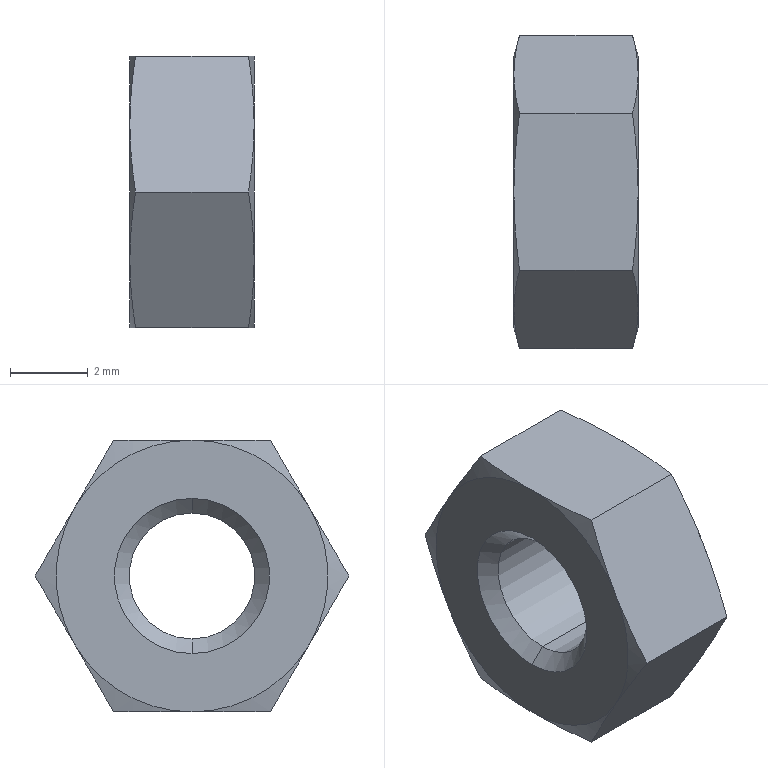Part | STEP file | 11-M4x0_7A11 | 1 solid | 26 faces | box 3.2 x 8.083 x 7 mm | volume 107.444 mm3 | cone 16 | plane 8 | cylinder 2 | commonest cylinder face diameters 3.242 x2
STEP:
#1=CARTESIAN_POINT('',(1.221,0.,-1.621));
#2=VERTEX_POINT('',#1);
#3=CARTESIAN_POINT('',(1.221,0.,1.621));
#4=VERTEX_POINT('',#3);
#5=CARTESIAN_POINT('',(1.221,0.,0.));
#6=DIRECTION('',(-1.,0.,0.));
#7=DIRECTION('',(0.,0.,1.));
#8=AXIS2_PLACEMENT_3D('',#5,#6,#7);
#9=CIRCLE('',#8,1.621);
#10=EDGE_CURVE('',#2,#4,#9,.T.);
#11=ORIENTED_EDGE('',*,*,#10,.T.);
#12=CARTESIAN_POINT('',(1.6,0.,2.));
#13=VERTEX_POINT('',#12);
#14=CARTESIAN_POINT('',(1.6,0.,2.));
#15=DIRECTION('',(0.7071,0.,0.7071));
#16=VECTOR('',#15,1000.);
#17=LINE('',#14,#16);
#18=EDGE_CURVE('',#4,#13,#17,.T.);
#19=ORIENTED_EDGE('',*,*,#18,.T.);
#20=CARTESIAN_POINT('',(1.6,0.,-2.));
#21=VERTEX_POINT('',#20);
#22=CARTESIAN_POINT('',(1.6,0.,0.));
#23=DIRECTION('',(-1.,0.,0.));
#24=DIRECTION('',(0.,0.,1.));
#25=AXIS2_PLACEMENT_3D('',#22,#23,#24);
#26=CIRCLE('',#25,2.);
#27=EDGE_CURVE('',#21,#13,#26,.T.);
#28=ORIENTED_EDGE('',*,*,#27,.F.);
#29=CARTESIAN_POINT('',(1.6,0.,-2.));
#30=DIRECTION('',(0.7071,0.,-0.7071));
#31=VECTOR('',#30,1000.);
#32=LINE('',#29,#31);
#33=EDGE_CURVE('',#2,#21,#32,.T.);
#34=ORIENTED_EDGE('',*,*,#33,.F.);
#35=EDGE_LOOP('',(#11,#19,#28,#34));
#36=FACE_OUTER_BOUND('',#35,.T.);
#37=CARTESIAN_POINT('',(1.6,0.,0.));
#38=DIRECTION('',(1.,0.,0.));
#39=DIRECTION('',(0.,0.,-1.));
#40=AXIS2_PLACEMENT_3D('',#37,#38,#39);
#41=CONICAL_SURFACE('',#40,2.,0.7854);
#42=ADVANCED_FACE('',(#36),#41,.F.);
#43=ORIENTED_EDGE('',*,*,#10,.F.);
#44=CARTESIAN_POINT('',(-1.221,0.,-1.621));
#45=VERTEX_POINT('',#44);
#46=CARTESIAN_POINT('',(1.6,0.,-1.621));
#47=DIRECTION('',(-1.,0.,0.));
#48=VECTOR('',#47,1000.);
#49=LINE('',#46,#48);
#50=EDGE_CURVE('',#2,#45,#49,.T.);
#51=ORIENTED_EDGE('',*,*,#50,.T.);
#52=CARTESIAN_POINT('',(-1.221,0.,1.621));
#53=VERTEX_POINT('',#52);
#54=CARTESIAN_POINT('',(-1.221,0.,0.));
#55=DIRECTION('',(-1.,0.,0.));
#56=DIRECTION('',(0.,0.,1.));
#57=AXIS2_PLACEMENT_3D('',#54,#55,#56);
#58=CIRCLE('',#57,1.621);
#59=EDGE_CURVE('',#45,#53,#58,.T.);
#60=ORIENTED_EDGE('',*,*,#59,.T.);
#61=CARTESIAN_POINT('',(1.6,0.,1.621));
#62=DIRECTION('',(-1.,0.,0.));
#63=VECTOR('',#62,1000.);
#64=LINE('',#61,#63);
#65=EDGE_CURVE('',#4,#53,#64,.T.);
#66=ORIENTED_EDGE('',*,*,#65,.F.);
#67=EDGE_LOOP('',(#43,#51,#60,#66));
#68=FACE_OUTER_BOUND('',#67,.T.);
#69=CARTESIAN_POINT('',(1.6,0.,0.));
#70=DIRECTION('',(-1.,0.,0.));
#71=DIRECTION('',(0.,0.,1.));
#72=AXIS2_PLACEMENT_3D('',#69,#70,#71);
#73=CYLINDRICAL_SURFACE('',#72,1.621);
#74=ADVANCED_FACE('',(#68),#73,.F.);
#75=ORIENTED_EDGE('',*,*,#59,.F.);
#76=CARTESIAN_POINT('',(-1.6,0.,-2.));
#77=VERTEX_POINT('',#76);
#78=CARTESIAN_POINT('',(-1.221,0.,-1.621));
#79=DIRECTION('',(-0.7071,0.,-0.7071));
#80=VECTOR('',#79,1000.);
#81=LINE('',#78,#80);
#82=EDGE_CURVE('',#45,#77,#81,.T.);
#83=ORIENTED_EDGE('',*,*,#82,.T.);
#84=CARTESIAN_POINT('',(-1.6,0.,2.));
#85=VERTEX_POINT('',#84);
#86=CARTESIAN_POINT('',(-1.6,0.,0.));
#87=DIRECTION('',(-1.,0.,0.));
#88=DIRECTION('',(0.,0.,1.));
#89=AXIS2_PLACEMENT_3D('',#86,#87,#88);
#90=CIRCLE('',#89,2.);
#91=EDGE_CURVE('',#77,#85,#90,.T.);
#92=ORIENTED_EDGE('',*,*,#91,.T.);
#93=CARTESIAN_POINT('',(-1.221,0.,1.621));
#94=DIRECTION('',(-0.7071,0.,0.7071));
#95=VECTOR('',#94,1000.);
#96=LINE('',#93,#95);
#97=EDGE_CURVE('',#53,#85,#96,.T.);
#98=ORIENTED_EDGE('',*,*,#97,.F.);
#99=EDGE_LOOP('',(#75,#83,#92,#98));
#100=FACE_OUTER_BOUND('',#99,.T.);
#101=CARTESIAN_POINT('',(-1.221,0.,0.));
#102=DIRECTION('',(-1.,0.,0.));
#103=DIRECTION('',(0.,0.,1.));
#104=AXIS2_PLACEMENT_3D('',#101,#102,#103);
#105=CONICAL_SURFACE('',#104,1.621,0.7854);
#106=ADVANCED_FACE('',(#100),#105,.F.);
#107=CARTESIAN_POINT('',(-1.6,-3.031,-1.75));
#108=VERTEX_POINT('',#107);
#109=CARTESIAN_POINT('',(-1.455,-4.041,0.));
#110=VERTEX_POINT('',#109);
#111=CARTESIAN_POINT('',(-1.6,-3.031,-1.75));
#112=CARTESIAN_POINT('',(-1.6,-3.368,-1.167));
#113=CARTESIAN_POINT('',(-1.545,-3.705,-0.5833));
#114=CARTESIAN_POINT('',(-1.455,-4.041,0.));
#115=B_SPLINE_CURVE_WITH_KNOTS('',3,(#111,#112,#113,#114),.UNSPECIFIED.,.F.,.F.,(4,4),(0.002021,0.004042),.UNSPECIFIED.);
#116=EDGE_CURVE('',#108,#110,#115,.T.);
#117=ORIENTED_EDGE('',*,*,#116,.T.);
#118=CARTESIAN_POINT('',(-1.6,-3.031,1.75));
#119=VERTEX_POINT('',#118);
#120=CARTESIAN_POINT('',(-1.455,-4.041,0.));
#121=CARTESIAN_POINT('',(-1.545,-3.705,0.5833));
#122=CARTESIAN_POINT('',(-1.6,-3.368,1.167));
#123=CARTESIAN_POINT('',(-1.6,-3.031,1.75));
#124=B_SPLINE_CURVE_WITH_KNOTS('',3,(#120,#121,#122,#123),.UNSPECIFIED.,.F.,.F.,(4,4),(0.000000231,0.002021),.UNSPECIFIED.);
#125=EDGE_CURVE('',#110,#119,#124,.T.);
#126=ORIENTED_EDGE('',*,*,#125,.T.);
#127=CARTESIAN_POINT('',(-1.6,0.,0.));
#128=DIRECTION('',(-1.,0.,0.));
#129=DIRECTION('',(0.,0.,1.));
#130=AXIS2_PLACEMENT_3D('',#127,#128,#129);
#131=CIRCLE('',#130,3.5);
#132=EDGE_CURVE('',#108,#119,#131,.T.);
#133=ORIENTED_EDGE('',*,*,#132,.F.);
#134=EDGE_LOOP('',(#117,#126,#133));
#135=FACE_OUTER_BOUND('',#134,.T.);
#136=CARTESIAN_POINT('',(-1.412,0.,0.));
#137=DIRECTION('',(1.,0.,0.));
#138=DIRECTION('',(0.,0.,-1.));
#139=AXIS2_PLACEMENT_3D('',#136,#137,#138);
#140=CONICAL_SURFACE('',#139,4.2,1.309);
#141=ADVANCED_FACE('',(#135),#140,.T.);
#142=CARTESIAN_POINT('',(-1.6,0.,3.5));
#143=VERTEX_POINT('',#142);
#144=CARTESIAN_POINT('',(-1.6,0.,0.));
#145=DIRECTION('',(-1.,0.,0.));
#146=DIRECTION('',(0.,0.,1.));
#147=AXIS2_PLACEMENT_3D('',#144,#145,#146);
#148=CIRCLE('',#147,3.5);
#149=EDGE_CURVE('',#119,#143,#148,.T.);
#150=ORIENTED_EDGE('',*,*,#149,.F.);
#151=CARTESIAN_POINT('',(-1.455,-2.021,3.5));
#152=VERTEX_POINT('',#151);
#153=CARTESIAN_POINT('',(-1.6,-3.031,1.75));
#154=CARTESIAN_POINT('',(-1.6,-2.694,2.333));
#155=CARTESIAN_POINT('',(-1.545,-2.358,2.917));
#156=CARTESIAN_POINT('',(-1.455,-2.021,3.5));
#157=B_SPLINE_CURVE_WITH_KNOTS('',3,(#153,#154,#155,#156),.UNSPECIFIED.,.F.,.F.,(4,4),(0.002021,0.004042),.UNSPECIFIED.);
#158=EDGE_CURVE('',#119,#152,#157,.T.);
#159=ORIENTED_EDGE('',*,*,#158,.T.);
#160=CARTESIAN_POINT('',(-1.455,-2.021,3.5));
#161=CARTESIAN_POINT('',(-1.545,-1.349,3.5));
#162=CARTESIAN_POINT('',(-1.6,-0.6726,3.5));
#163=CARTESIAN_POINT('',(-1.6,0.,3.5));
#164=B_SPLINE_CURVE_WITH_KNOTS('',3,(#160,#161,#162,#163),.UNSPECIFIED.,.F.,.F.,(4,4),(0.003384,0.005414),.UNSPECIFIED.);
#165=EDGE_CURVE('',#152,#143,#164,.T.);
#166=ORIENTED_EDGE('',*,*,#165,.T.);
#167=EDGE_LOOP('',(#150,#159,#166));
#168=FACE_OUTER_BOUND('',#167,.T.);
#169=CARTESIAN_POINT('',(-1.412,0.,0.));
#170=DIRECTION('',(1.,0.,0.));
#171=DIRECTION('',(0.,0.,-1.));
#172=AXIS2_PLACEMENT_3D('',#169,#170,#171);
#173=CONICAL_SURFACE('',#172,4.2,1.309);
#174=ADVANCED_FACE('',(#168),#173,.T.);
#175=CARTESIAN_POINT('',(-1.6,3.031,1.75));
#176=VERTEX_POINT('',#175);
#177=CARTESIAN_POINT('',(-1.6,0.,0.));
#178=DIRECTION('',(-1.,0.,0.));
#179=DIRECTION('',(0.,0.,1.));
#180=AXIS2_PLACEMENT_3D('',#177,#178,#179);
#181=CIRCLE('',#180,3.5);
#182=EDGE_CURVE('',#143,#176,#181,.T.);
#183=ORIENTED_EDGE('',*,*,#182,.F.);
#184=CARTESIAN_POINT('',(-1.455,2.021,3.5));
#185=VERTEX_POINT('',#184);
#186=CARTESIAN_POINT('',(-1.6,0.,3.5));
#187=CARTESIAN_POINT('',(-1.6,0.675,3.5));
#188=CARTESIAN_POINT('',(-1.545,1.348,3.5));
#189=CARTESIAN_POINT('',(-1.455,2.021,3.5));
#190=B_SPLINE_CURVE_WITH_KNOTS('',3,(#186,#187,#188,#189),.UNSPECIFIED.,.F.,.F.,(4,4),(0.005414,0.007452),.UNSPECIFIED.);
#191=EDGE_CURVE('',#143,#185,#190,.T.);
#192=ORIENTED_EDGE('',*,*,#191,.T.);
#193=CARTESIAN_POINT('',(-1.455,2.021,3.5));
#194=CARTESIAN_POINT('',(-1.545,2.358,2.917));
#195=CARTESIAN_POINT('',(-1.6,2.694,2.333));
#196=CARTESIAN_POINT('',(-1.6,3.031,1.75));
#197=B_SPLINE_CURVE_WITH_KNOTS('',3,(#193,#194,#195,#196),.UNSPECIFIED.,.F.,.F.,(4,4),(0.000000231,0.002021),.UNSPECIFIED.);
#198=EDGE_CURVE('',#185,#176,#197,.T.);
#199=ORIENTED_EDGE('',*,*,#198,.T.);
#200=EDGE_LOOP('',(#183,#192,#199));
#201=FACE_OUTER_BOUND('',#200,.T.);
#202=CARTESIAN_POINT('',(-1.412,0.,0.));
#203=DIRECTION('',(1.,0.,0.));
#204=DIRECTION('',(0.,0.,-1.));
#205=AXIS2_PLACEMENT_3D('',#202,#203,#204);
#206=CONICAL_SURFACE('',#205,4.2,1.309);
#207=ADVANCED_FACE('',(#201),#206,.T.);
#208=CARTESIAN_POINT('',(-1.6,0.,-3.5));
#209=VERTEX_POINT('',#208);
#210=CARTESIAN_POINT('',(-1.455,-2.021,-3.5));
#211=VERTEX_POINT('',#210);
#212=CARTESIAN_POINT('',(-1.6,0.,-3.5));
#213=CARTESIAN_POINT('',(-1.6,-0.6726,-3.5));
#214=CARTESIAN_POINT('',(-1.545,-1.349,-3.5));
#215=CARTESIAN_POINT('',(-1.455,-2.021,-3.5));
#216=B_SPLINE_CURVE_WITH_KNOTS('',3,(#212,#213,#214,#215),.UNSPECIFIED.,.F.,.F.,(4,4),(0.009728,0.01176),.UNSPECIFIED.);
#217=EDGE_CURVE('',#209,#211,#216,.T.);
#218=ORIENTED_EDGE('',*,*,#217,.T.);
#219=CARTESIAN_POINT('',(-1.455,-2.021,-3.5));
#220=CARTESIAN_POINT('',(-1.545,-2.358,-2.917));
#221=CARTESIAN_POINT('',(-1.6,-2.694,-2.333));
#222=CARTESIAN_POINT('',(-1.6,-3.031,-1.75));
#223=B_SPLINE_CURVE_WITH_KNOTS('',3,(#219,#220,#221,#222),.UNSPECIFIED.,.F.,.F.,(4,4),(0.000000231,0.002021),.UNSPECIFIED.);
#224=EDGE_CURVE('',#211,#108,#223,.T.);
#225=ORIENTED_EDGE('',*,*,#224,.T.);
#226=CARTESIAN_POINT('',(-1.6,0.,0.));
#227=DIRECTION('',(-1.,0.,0.));
#228=DIRECTION('',(0.,0.,1.));
#229=AXIS2_PLACEMENT_3D('',#226,#227,#228);
#230=CIRCLE('',#229,3.5);
#231=EDGE_CURVE('',#209,#108,#230,.T.);
#232=ORIENTED_EDGE('',*,*,#231,.F.);
#233=EDGE_LOOP('',(#218,#225,#232));
#234=FACE_OUTER_BOUND('',#233,.T.);
#235=CARTESIAN_POINT('',(-1.412,0.,0.));
#236=DIRECTION('',(1.,0.,0.));
#237=DIRECTION('',(0.,0.,-1.));
#238=AXIS2_PLACEMENT_3D('',#235,#236,#237);
#239=CONICAL_SURFACE('',#238,4.2,1.309);
#240=ADVANCED_FACE('',(#234),#239,.T.);
#241=CARTESIAN_POINT('',(-1.6,3.031,-1.75));
#242=VERTEX_POINT('',#241);
#243=CARTESIAN_POINT('',(-1.6,0.,0.));
#244=DIRECTION('',(-1.,0.,0.));
#245=DIRECTION('',(0.,0.,1.));
#246=AXIS2_PLACEMENT_3D('',#243,#244,#245);
#247=CIRCLE('',#246,3.5);
#248=EDGE_CURVE('',#176,#242,#247,.T.);
#249=ORIENTED_EDGE('',*,*,#248,.F.);
#250=CARTESIAN_POINT('',(-1.455,4.041,0.));
#251=VERTEX_POINT('',#250);
#252=CARTESIAN_POINT('',(-1.6,3.031,1.75));
#253=CARTESIAN_POINT('',(-1.6,3.368,1.167));
#254=CARTESIAN_POINT('',(-1.545,3.705,0.5833));
#255=CARTESIAN_POINT('',(-1.455,4.041,0.));
#256=B_SPLINE_CURVE_WITH_KNOTS('',3,(#252,#253,#254,#255),.UNSPECIFIED.,.F.,.F.,(4,4),(0.002021,0.004042),.UNSPECIFIED.);
#257=EDGE_CURVE('',#176,#251,#256,.T.);
#258=ORIENTED_EDGE('',*,*,#257,.T.);
#259=CARTESIAN_POINT('',(-1.455,4.041,0.));
#260=CARTESIAN_POINT('',(-1.545,3.705,-0.5833));
#261=CARTESIAN_POINT('',(-1.6,3.368,-1.167));
#262=CARTESIAN_POINT('',(-1.6,3.031,-1.75));
#263=B_SPLINE_CURVE_WITH_KNOTS('',3,(#259,#260,#261,#262),.UNSPECIFIED.,.F.,.F.,(4,4),(0.000000231,0.002021),.UNSPECIFIED.);
#264=EDGE_CURVE('',#251,#242,#263,.T.);
#265=ORIENTED_EDGE('',*,*,#264,.T.);
#266=EDGE_LOOP('',(#249,#258,#265));
#267=FACE_OUTER_BOUND('',#266,.T.);
#268=CARTESIAN_POINT('',(-1.412,0.,0.));
#269=DIRECTION('',(1.,0.,0.));
#270=DIRECTION('',(0.,0.,-1.));
#271=AXIS2_PLACEMENT_3D('',#268,#269,#270);
#272=CONICAL_SURFACE('',#271,4.2,1.309);
#273=ADVANCED_FACE('',(#267),#272,.T.);
#274=CARTESIAN_POINT('',(1.6,3.031,-1.75));
#275=VERTEX_POINT('',#274);
#276=CARTESIAN_POINT('',(1.455,4.041,0.));
#277=VERTEX_POINT('',#276);
#278=CARTESIAN_POINT('',(1.6,3.031,-1.75));
#279=CARTESIAN_POINT('',(1.6,3.368,-1.167));
#280=CARTESIAN_POINT('',(1.545,3.705,-0.5833));
#281=CARTESIAN_POINT('',(1.455,4.041,0.));
#282=B_SPLINE_CURVE_WITH_KNOTS('',3,(#278,#279,#280,#281),.UNSPECIFIED.,.F.,.F.,(4,4),(0.002021,0.004042),.UNSPECIFIED.);
#283=EDGE_CURVE('',#275,#277,#282,.T.);
#284=ORIENTED_EDGE('',*,*,#283,.T.);
#285=CARTESIAN_POINT('',(1.6,3.031,1.75));
#286=VERTEX_POINT('',#285);
#287=CARTESIAN_POINT('',(1.455,4.041,0.));
#288=CARTESIAN_POINT('',(1.545,3.705,0.5833));
#289=CARTESIAN_POINT('',(1.6,3.368,1.167));
#290=CARTESIAN_POINT('',(1.6,3.031,1.75));
#291=B_SPLINE_CURVE_WITH_KNOTS('',3,(#287,#288,#289,#290),.UNSPECIFIED.,.F.,.F.,(4,4),(0.000000231,0.002021),.UNSPECIFIED.);
#292=EDGE_CURVE('',#277,#286,#291,.T.);
#293=ORIENTED_EDGE('',*,*,#292,.T.);
#294=CARTESIAN_POINT('',(1.6,0.,0.));
#295=DIRECTION('',(-1.,0.,0.));
#296=DIRECTION('',(0.,0.,1.));
#297=AXIS2_PLACEMENT_3D('',#294,#295,#296);
#298=CIRCLE('',#297,3.5);
#299=EDGE_CURVE('',#286,#275,#298,.T.);
#300=ORIENTED_EDGE('',*,*,#299,.T.);
#301=EDGE_LOOP('',(#284,#293,#300));
#302=FACE_OUTER_BOUND('',#301,.T.);
#303=CARTESIAN_POINT('',(1.6,0.,0.));
#304=DIRECTION('',(-1.,0.,0.));
#305=DIRECTION('',(0.,0.,1.));
#306=AXIS2_PLACEMENT_3D('',#303,#304,#305);
#307=CONICAL_SURFACE('',#306,3.5,1.309);
#308=ADVANCED_FACE('',(#302),#307,.T.);
#309=CARTESIAN_POINT('',(1.6,0.,3.5));
#310=VERTEX_POINT('',#309);
#311=CARTESIAN_POINT('',(1.6,0.,0.));
#312=DIRECTION('',(-1.,0.,0.));
#313=DIRECTION('',(0.,0.,1.));
#314=AXIS2_PLACEMENT_3D('',#311,#312,#313);
#315=CIRCLE('',#314,3.5);
#316=EDGE_CURVE('',#310,#286,#315,.T.);
#317=ORIENTED_EDGE('',*,*,#316,.T.);
#318=CARTESIAN_POINT('',(1.455,2.021,3.5));
#319=VERTEX_POINT('',#318);
#320=CARTESIAN_POINT('',(1.6,3.031,1.75));
#321=CARTESIAN_POINT('',(1.6,2.694,2.333));
#322=CARTESIAN_POINT('',(1.545,2.358,2.917));
#323=CARTESIAN_POINT('',(1.455,2.021,3.5));
#324=B_SPLINE_CURVE_WITH_KNOTS('',3,(#320,#321,#322,#323),.UNSPECIFIED.,.F.,.F.,(4,4),(0.002021,0.004042),.UNSPECIFIED.);
#325=EDGE_CURVE('',#286,#319,#324,.T.);
#326=ORIENTED_EDGE('',*,*,#325,.T.);
#327=CARTESIAN_POINT('',(1.455,2.021,3.5));
#328=CARTESIAN_POINT('',(1.545,1.348,3.5));
#329=CARTESIAN_POINT('',(1.6,0.675,3.5));
#330=CARTESIAN_POINT('',(1.6,0.,3.5));
#331=B_SPLINE_CURVE_WITH_KNOTS('',3,(#327,#328,#329,#330),.UNSPECIFIED.,.F.,.F.,(4,4),(0.007694,0.009728),.UNSPECIFIED.);
#332=EDGE_CURVE('',#319,#310,#331,.T.);
#333=ORIENTED_EDGE('',*,*,#332,.T.);
#334=EDGE_LOOP('',(#317,#326,#333));
#335=FACE_OUTER_BOUND('',#334,.T.);
#336=CARTESIAN_POINT('',(1.6,0.,0.));
#337=DIRECTION('',(-1.,0.,0.));
#338=DIRECTION('',(0.,0.,1.));
#339=AXIS2_PLACEMENT_3D('',#336,#337,#338);
#340=CONICAL_SURFACE('',#339,3.5,1.309);
#341=ADVANCED_FACE('',(#335),#340,.T.);
#342=CARTESIAN_POINT('',(1.6,-3.031,1.75));
#343=VERTEX_POINT('',#342);
#344=CARTESIAN_POINT('',(1.6,0.,0.));
#345=DIRECTION('',(-1.,0.,0.));
#346=DIRECTION('',(0.,0.,1.));
#347=AXIS2_PLACEMENT_3D('',#344,#345,#346);
#348=CIRCLE('',#347,3.5);
#349=EDGE_CURVE('',#343,#310,#348,.T.);
#350=ORIENTED_EDGE('',*,*,#349,.T.);
#351=CARTESIAN_POINT('',(1.455,-2.021,3.5));
#352=VERTEX_POINT('',#351);
#353=CARTESIAN_POINT('',(1.6,0.,3.5));
#354=CARTESIAN_POINT('',(1.6,-0.6726,3.5));
#355=CARTESIAN_POINT('',(1.545,-1.349,3.5));
#356=CARTESIAN_POINT('',(1.455,-2.021,3.5));
#357=B_SPLINE_CURVE_WITH_KNOTS('',3,(#353,#354,#355,#356),.UNSPECIFIED.,.F.,.F.,(4,4),(0.009728,0.01176),.UNSPECIFIED.);
#358=EDGE_CURVE('',#310,#352,#357,.T.);
#359=ORIENTED_EDGE('',*,*,#358,.T.);
#360=CARTESIAN_POINT('',(1.455,-2.021,3.5));
#361=CARTESIAN_POINT('',(1.545,-2.358,2.917));
#362=CARTESIAN_POINT('',(1.6,-2.694,2.333));
#363=CARTESIAN_POINT('',(1.6,-3.031,1.75));
#364=B_SPLINE_CURVE_WITH_KNOTS('',3,(#360,#361,#362,#363),.UNSPECIFIED.,.F.,.F.,(4,4),(0.000000231,0.002021),.UNSPECIFIED.);
#365=EDGE_CURVE('',#352,#343,#364,.T.);
#366=ORIENTED_EDGE('',*,*,#365,.T.);
#367=EDGE_LOOP('',(#350,#359,#366));
#368=FACE_OUTER_BOUND('',#367,.T.);
#369=CARTESIAN_POINT('',(1.6,0.,0.));
#370=DIRECTION('',(-1.,0.,0.));
#371=DIRECTION('',(0.,0.,1.));
#372=AXIS2_PLACEMENT_3D('',#369,#370,#371);
#373=CONICAL_SURFACE('',#372,3.5,1.309);
#374=ADVANCED_FACE('',(#368),#373,.T.);
#375=CARTESIAN_POINT('',(1.6,-3.031,-1.75));
#376=VERTEX_POINT('',#375);
#377=CARTESIAN_POINT('',(1.6,0.,0.));
#378=DIRECTION('',(-1.,0.,0.));
#379=DIRECTION('',(0.,0.,1.));
#380=AXIS2_PLACEMENT_3D('',#377,#378,#379);
#381=CIRCLE('',#380,3.5);
#382=EDGE_CURVE('',#376,#343,#381,.T.);
#383=ORIENTED_EDGE('',*,*,#382,.T.);
#384=CARTESIAN_POINT('',(1.455,-4.041,0.));
#385=VERTEX_POINT('',#384);
#386=CARTESIAN_POINT('',(1.6,-3.031,1.75));
#387=CARTESIAN_POINT('',(1.6,-3.368,1.167));
#388=CARTESIAN_POINT('',(1.545,-3.705,0.5833));
#389=CARTESIAN_POINT('',(1.455,-4.041,0.));
#390=B_SPLINE_CURVE_WITH_KNOTS('',3,(#386,#387,#388,#389),.UNSPECIFIED.,.F.,.F.,(4,4),(0.002021,0.004042),.UNSPECIFIED.);
#391=EDGE_CURVE('',#343,#385,#390,.T.);
#392=ORIENTED_EDGE('',*,*,#391,.T.);
#393=CARTESIAN_POINT('',(1.455,-4.041,0.));
#394=CARTESIAN_POINT('',(1.545,-3.705,-0.5833));
#395=CARTESIAN_POINT('',(1.6,-3.368,-1.167));
#396=CARTESIAN_POINT('',(1.6,-3.031,-1.75));
#397=B_SPLINE_CURVE_WITH_KNOTS('',3,(#393,#394,#395,#396),.UNSPECIFIED.,.F.,.F.,(4,4),(0.000000231,0.002021),.UNSPECIFIED.);
#398=EDGE_CURVE('',#385,#376,#397,.T.);
#399=ORIENTED_EDGE('',*,*,#398,.T.);
#400=EDGE_LOOP('',(#383,#392,#399));
#401=FACE_OUTER_BOUND('',#400,.T.);
#402=CARTESIAN_POINT('',(1.6,0.,0.));
#403=DIRECTION('',(-1.,0.,0.));
#404=DIRECTION('',(0.,0.,1.));
#405=AXIS2_PLACEMENT_3D('',#402,#403,#404);
#406=CONICAL_SURFACE('',#405,3.5,1.309);
#407=ADVANCED_FACE('',(#401),#406,.T.);
#408=CARTESIAN_POINT('',(1.6,0.,-3.5));
#409=VERTEX_POINT('',#408);
#410=CARTESIAN_POINT('',(1.6,0.,0.));
#411=DIRECTION('',(-1.,0.,0.));
#412=DIRECTION('',(0.,0.,1.));
#413=AXIS2_PLACEMENT_3D('',#410,#411,#412);
#414=CIRCLE('',#413,3.5);
#415=EDGE_CURVE('',#409,#376,#414,.T.);
#416=ORIENTED_EDGE('',*,*,#415,.T.);
#417=CARTESIAN_POINT('',(1.455,-2.021,-3.5));
#418=VERTEX_POINT('',#417);
#419=CARTESIAN_POINT('',(1.6,-3.031,-1.75));
#420=CARTESIAN_POINT('',(1.6,-2.694,-2.333));
#421=CARTESIAN_POINT('',(1.545,-2.358,-2.917));
#422=CARTESIAN_POINT('',(1.455,-2.021,-3.5));
#423=B_SPLINE_CURVE_WITH_KNOTS('',3,(#419,#420,#421,#422),.UNSPECIFIED.,.F.,.F.,(4,4),(0.002021,0.004042),.UNSPECIFIED.);
#424=EDGE_CURVE('',#376,#418,#423,.T.);
#425=ORIENTED_EDGE('',*,*,#424,.T.);
#426=CARTESIAN_POINT('',(1.455,-2.021,-3.5));
#427=CARTESIAN_POINT('',(1.545,-1.349,-3.5));
#428=CARTESIAN_POINT('',(1.6,-0.6726,-3.5));
#429=CARTESIAN_POINT('',(1.6,0.,-3.5));
#430=B_SPLINE_CURVE_WITH_KNOTS('',3,(#426,#427,#428,#429),.UNSPECIFIED.,.F.,.F.,(4,4),(0.003384,0.005414),.UNSPECIFIED.);
#431=EDGE_CURVE('',#418,#409,#430,.T.);
#432=ORIENTED_EDGE('',*,*,#431,.T.);
#433=EDGE_LOOP('',(#416,#425,#432));
#434=FACE_OUTER_BOUND('',#433,.T.);
#435=CARTESIAN_POINT('',(1.6,0.,0.));
#436=DIRECTION('',(-1.,0.,0.));
#437=DIRECTION('',(0.,0.,1.));
#438=AXIS2_PLACEMENT_3D('',#435,#436,#437);
#439=CONICAL_SURFACE('',#438,3.5,1.309);
#440=ADVANCED_FACE('',(#434),#439,.T.);
#441=ORIENTED_EDGE('',*,*,#182,.T.);
#442=ORIENTED_EDGE('',*,*,#248,.T.);
#443=CARTESIAN_POINT('',(-1.6,0.,0.));
#444=DIRECTION('',(-1.,0.,0.));
#445=DIRECTION('',(0.,0.,1.));
#446=AXIS2_PLACEMENT_3D('',#443,#444,#445);
#447=CIRCLE('',#446,3.5);
#448=EDGE_CURVE('',#242,#209,#447,.T.);
#449=ORIENTED_EDGE('',*,*,#448,.T.);
#450=ORIENTED_EDGE('',*,*,#231,.T.);
#451=ORIENTED_EDGE('',*,*,#132,.T.);
#452=ORIENTED_EDGE('',*,*,#149,.T.);
#453=EDGE_LOOP('',(#441,#442,#449,#450,#451,#452));
#454=FACE_OUTER_BOUND('',#453,.T.);
#455=CARTESIAN_POINT('',(-1.6,0.,0.));
#456=DIRECTION('',(-1.,0.,0.));
#457=DIRECTION('',(0.,0.,1.));
#458=AXIS2_PLACEMENT_3D('',#455,#456,#457);
#459=CIRCLE('',#458,2.);
#460=EDGE_CURVE('',#85,#77,#459,.T.);
#461=ORIENTED_EDGE('',*,*,#460,.F.);
#462=ORIENTED_EDGE('',*,*,#91,.F.);
#463=EDGE_LOOP('',(#461,#462));
#464=FACE_BOUND('',#463,.T.);
#465=CARTESIAN_POINT('',(-1.6,0.,0.));
#466=DIRECTION('',(1.,0.,0.));
#467=DIRECTION('',(0.,0.,-1.));
#468=AXIS2_PLACEMENT_3D('',#465,#466,#467);
#469=PLANE('',#468);
#470=ADVANCED_FACE('',(#454,#464),#469,.F.);
#471=ORIENTED_EDGE('',*,*,#316,.F.);
#472=ORIENTED_EDGE('',*,*,#349,.F.);
#473=ORIENTED_EDGE('',*,*,#382,.F.);
#474=ORIENTED_EDGE('',*,*,#415,.F.);
#475=CARTESIAN_POINT('',(1.6,0.,0.));
#476=DIRECTION('',(-1.,0.,0.));
#477=DIRECTION('',(0.,0.,1.));
#478=AXIS2_PLACEMENT_3D('',#475,#476,#477);
#479=CIRCLE('',#478,3.5);
#480=EDGE_CURVE('',#275,#409,#479,.T.);
#481=ORIENTED_EDGE('',*,*,#480,.F.);
#482=ORIENTED_EDGE('',*,*,#299,.F.);
#483=EDGE_LOOP('',(#471,#472,#473,#474,#481,#482));
#484=FACE_OUTER_BOUND('',#483,.T.);
#485=ORIENTED_EDGE('',*,*,#27,.T.);
#486=CARTESIAN_POINT('',(1.6,0.,0.));
#487=DIRECTION('',(-1.,0.,0.));
#488=DIRECTION('',(0.,0.,1.));
#489=AXIS2_PLACEMENT_3D('',#486,#487,#488);
#490=CIRCLE('',#489,2.);
#491=EDGE_CURVE('',#13,#21,#490,.T.);
#492=ORIENTED_EDGE('',*,*,#491,.T.);
#493=EDGE_LOOP('',(#485,#492));
#494=FACE_BOUND('',#493,.T.);
#495=CARTESIAN_POINT('',(1.6,3.5,0.));
#496=DIRECTION('',(-1.,0.,0.));
#497=DIRECTION('',(0.,0.,1.));
#498=AXIS2_PLACEMENT_3D('',#495,#496,#497);
#499=PLANE('',#498);
#500=ADVANCED_FACE('',(#484,#494),#499,.F.);
#501=CARTESIAN_POINT('',(-1.455,2.021,-3.5));
#502=VERTEX_POINT('',#501);
#503=CARTESIAN_POINT('',(-1.6,3.031,-1.75));
#504=CARTESIAN_POINT('',(-1.6,2.694,-2.333));
#505=CARTESIAN_POINT('',(-1.545,2.358,-2.917));
#506=CARTESIAN_POINT('',(-1.455,2.021,-3.5));
#507=B_SPLINE_CURVE_WITH_KNOTS('',3,(#503,#504,#505,#506),.UNSPECIFIED.,.F.,.F.,(4,4),(0.002021,0.004042),.UNSPECIFIED.);
#508=EDGE_CURVE('',#242,#502,#507,.T.);
#509=ORIENTED_EDGE('',*,*,#508,.T.);
#510=CARTESIAN_POINT('',(-1.455,2.021,-3.5));
#511=CARTESIAN_POINT('',(-1.545,1.348,-3.5));
#512=CARTESIAN_POINT('',(-1.6,0.675,-3.5));
#513=CARTESIAN_POINT('',(-1.6,0.,-3.5));
#514=B_SPLINE_CURVE_WITH_KNOTS('',3,(#510,#511,#512,#513),.UNSPECIFIED.,.F.,.F.,(4,4),(0.007694,0.009728),.UNSPECIFIED.);
#515=EDGE_CURVE('',#502,#209,#514,.T.);
#516=ORIENTED_EDGE('',*,*,#515,.T.);
#517=ORIENTED_EDGE('',*,*,#448,.F.);
#518=EDGE_LOOP('',(#509,#516,#517));
#519=FACE_OUTER_BOUND('',#518,.T.);
#520=CARTESIAN_POINT('',(-1.412,0.,0.));
#521=DIRECTION('',(1.,0.,0.));
#522=DIRECTION('',(0.,0.,-1.));
#523=AXIS2_PLACEMENT_3D('',#520,#521,#522);
#524=CONICAL_SURFACE('',#523,4.2,1.309);
#525=ADVANCED_FACE('',(#519),#524,.T.);
#526=ORIENTED_EDGE('',*,*,#480,.T.);
#527=CARTESIAN_POINT('',(1.455,2.021,-3.5));
#528=VERTEX_POINT('',#527);
#529=CARTESIAN_POINT('',(1.6,0.,-3.5));
#530=CARTESIAN_POINT('',(1.6,0.675,-3.5));
#531=CARTESIAN_POINT('',(1.545,1.348,-3.5));
#532=CARTESIAN_POINT('',(1.455,2.021,-3.5));
#533=B_SPLINE_CURVE_WITH_KNOTS('',3,(#529,#530,#531,#532),.UNSPECIFIED.,.F.,.F.,(4,4),(0.005414,0.007452),.UNSPECIFIED.);
#534=EDGE_CURVE('',#409,#528,#533,.T.);
#535=ORIENTED_EDGE('',*,*,#534,.T.);
#536=CARTESIAN_POINT('',(1.455,2.021,-3.5));
#537=CARTESIAN_POINT('',(1.545,2.358,-2.917));
#538=CARTESIAN_POINT('',(1.6,2.694,-2.333));
#539=CARTESIAN_POINT('',(1.6,3.031,-1.75));
#540=B_SPLINE_CURVE_WITH_KNOTS('',3,(#536,#537,#538,#539),.UNSPECIFIED.,.F.,.F.,(4,4),(0.000000231,0.002021),.UNSPECIFIED.);
#541=EDGE_CURVE('',#528,#275,#540,.T.);
#542=ORIENTED_EDGE('',*,*,#541,.T.);
#543=EDGE_LOOP('',(#526,#535,#542));
#544=FACE_OUTER_BOUND('',#543,.T.);
#545=CARTESIAN_POINT('',(1.6,0.,0.));
#546=DIRECTION('',(-1.,0.,0.));
#547=DIRECTION('',(0.,0.,1.));
#548=AXIS2_PLACEMENT_3D('',#545,#546,#547);
#549=CONICAL_SURFACE('',#548,3.5,1.309);
#550=ADVANCED_FACE('',(#544),#549,.T.);
#551=ORIENTED_EDGE('',*,*,#82,.F.);
#552=CARTESIAN_POINT('',(-1.221,0.,0.));
#553=DIRECTION('',(-1.,0.,0.));
#554=DIRECTION('',(0.,0.,1.));
#555=AXIS2_PLACEMENT_3D('',#552,#553,#554);
#556=CIRCLE('',#555,1.621);
#557=EDGE_CURVE('',#53,#45,#556,.T.);
#558=ORIENTED_EDGE('',*,*,#557,.F.);
#559=ORIENTED_EDGE('',*,*,#97,.T.);
#560=ORIENTED_EDGE('',*,*,#460,.T.);
#561=EDGE_LOOP('',(#551,#558,#559,#560));
#562=FACE_OUTER_BOUND('',#561,.T.);
#563=CARTESIAN_POINT('',(-1.221,0.,0.));
#564=DIRECTION('',(-1.,0.,0.));
#565=DIRECTION('',(0.,0.,1.));
#566=AXIS2_PLACEMENT_3D('',#563,#564,#565);
#567=CONICAL_SURFACE('',#566,1.621,0.7854);
#568=ADVANCED_FACE('',(#562),#567,.F.);
#569=ORIENTED_EDGE('',*,*,#50,.F.);
#570=CARTESIAN_POINT('',(1.221,0.,0.));
#571=DIRECTION('',(-1.,0.,0.));
#572=DIRECTION('',(0.,0.,1.));
#573=AXIS2_PLACEMENT_3D('',#570,#571,#572);
#574=CIRCLE('',#573,1.621);
#575=EDGE_CURVE('',#4,#2,#574,.T.);
#576=ORIENTED_EDGE('',*,*,#575,.F.);
#577=ORIENTED_EDGE('',*,*,#65,.T.);
#578=ORIENTED_EDGE('',*,*,#557,.T.);
#579=EDGE_LOOP('',(#569,#576,#577,#578));
#580=FACE_OUTER_BOUND('',#579,.T.);
#581=CARTESIAN_POINT('',(1.6,0.,0.));
#582=DIRECTION('',(-1.,0.,0.));
#583=DIRECTION('',(0.,0.,1.));
#584=AXIS2_PLACEMENT_3D('',#581,#582,#583);
#585=CYLINDRICAL_SURFACE('',#584,1.621);
#586=ADVANCED_FACE('',(#580),#585,.F.);
#587=ORIENTED_EDGE('',*,*,#18,.F.);
#588=ORIENTED_EDGE('',*,*,#575,.T.);
#589=ORIENTED_EDGE('',*,*,#33,.T.);
#590=ORIENTED_EDGE('',*,*,#491,.F.);
#591=EDGE_LOOP('',(#587,#588,#589,#590));
#592=FACE_OUTER_BOUND('',#591,.T.);
#593=CARTESIAN_POINT('',(1.6,0.,0.));
#594=DIRECTION('',(1.,0.,0.));
#595=DIRECTION('',(0.,0.,-1.));
#596=AXIS2_PLACEMENT_3D('',#593,#594,#595);
#597=CONICAL_SURFACE('',#596,2.,0.7854);
#598=ADVANCED_FACE('',(#592),#597,.F.);
#599=CARTESIAN_POINT('',(3.2,2.021,3.5));
#600=DIRECTION('',(-1.,0.,0.));
#601=VECTOR('',#600,1000.);
#602=LINE('',#599,#601);
#603=EDGE_CURVE('',#319,#185,#602,.T.);
#604=ORIENTED_EDGE('',*,*,#603,.F.);
#605=ORIENTED_EDGE('',*,*,#325,.F.);
#606=ORIENTED_EDGE('',*,*,#292,.F.);
#607=CARTESIAN_POINT('',(3.2,4.041,0.));
#608=DIRECTION('',(-1.,0.,0.));
#609=VECTOR('',#608,1000.);
#610=LINE('',#607,#609);
#611=EDGE_CURVE('',#277,#251,#610,.T.);
#612=ORIENTED_EDGE('',*,*,#611,.T.);
#613=ORIENTED_EDGE('',*,*,#257,.F.);
#614=ORIENTED_EDGE('',*,*,#198,.F.);
#615=EDGE_LOOP('',(#604,#605,#606,#612,#613,#614));
#616=FACE_OUTER_BOUND('',#615,.T.);
#617=CARTESIAN_POINT('',(3.2,4.041,0.));
#618=DIRECTION('',(0.,-0.866,-0.5));
#619=DIRECTION('',(0.,0.5,-0.866));
#620=AXIS2_PLACEMENT_3D('',#617,#618,#619);
#621=PLANE('',#620);
#622=ADVANCED_FACE('',(#616),#621,.F.);
#623=CARTESIAN_POINT('',(3.2,-2.021,3.5));
#624=DIRECTION('',(-1.,0.,0.));
#625=VECTOR('',#624,1000.);
#626=LINE('',#623,#625);
#627=EDGE_CURVE('',#352,#152,#626,.T.);
#628=ORIENTED_EDGE('',*,*,#627,.F.);
#629=ORIENTED_EDGE('',*,*,#358,.F.);
#630=ORIENTED_EDGE('',*,*,#332,.F.);
#631=ORIENTED_EDGE('',*,*,#603,.T.);
#632=ORIENTED_EDGE('',*,*,#191,.F.);
#633=ORIENTED_EDGE('',*,*,#165,.F.);
#634=EDGE_LOOP('',(#628,#629,#630,#631,#632,#633));
#635=FACE_OUTER_BOUND('',#634,.T.);
#636=CARTESIAN_POINT('',(3.2,2.021,3.5));
#637=DIRECTION('',(0.,0.,-1.));
#638=DIRECTION('',(-1.,0.,0.));
#639=AXIS2_PLACEMENT_3D('',#636,#637,#638);
#640=PLANE('',#639);
#641=ADVANCED_FACE('',(#635),#640,.F.);
#642=CARTESIAN_POINT('',(3.2,-4.041,0.));
#643=DIRECTION('',(-1.,0.,0.));
#644=VECTOR('',#643,1000.);
#645=LINE('',#642,#644);
#646=EDGE_CURVE('',#385,#110,#645,.T.);
#647=ORIENTED_EDGE('',*,*,#646,.F.);
#648=ORIENTED_EDGE('',*,*,#391,.F.);
#649=ORIENTED_EDGE('',*,*,#365,.F.);
#650=ORIENTED_EDGE('',*,*,#627,.T.);
#651=ORIENTED_EDGE('',*,*,#158,.F.);
#652=ORIENTED_EDGE('',*,*,#125,.F.);
#653=EDGE_LOOP('',(#647,#648,#649,#650,#651,#652));
#654=FACE_OUTER_BOUND('',#653,.T.);
#655=CARTESIAN_POINT('',(3.2,-2.021,3.5));
#656=DIRECTION('',(0.,0.866,-0.5));
#657=DIRECTION('',(0.,0.5,0.866));
#658=AXIS2_PLACEMENT_3D('',#655,#656,#657);
#659=PLANE('',#658);
#660=ADVANCED_FACE('',(#654),#659,.F.);
#661=CARTESIAN_POINT('',(3.2,-2.021,-3.5));
#662=DIRECTION('',(-1.,0.,0.));
#663=VECTOR('',#662,1000.);
#664=LINE('',#661,#663);
#665=EDGE_CURVE('',#418,#211,#664,.T.);
#666=ORIENTED_EDGE('',*,*,#665,.F.);
#667=ORIENTED_EDGE('',*,*,#424,.F.);
#668=ORIENTED_EDGE('',*,*,#398,.F.);
#669=ORIENTED_EDGE('',*,*,#646,.T.);
#670=ORIENTED_EDGE('',*,*,#116,.F.);
#671=ORIENTED_EDGE('',*,*,#224,.F.);
#672=EDGE_LOOP('',(#666,#667,#668,#669,#670,#671));
#673=FACE_OUTER_BOUND('',#672,.T.);
#674=CARTESIAN_POINT('',(3.2,-4.041,0.));
#675=DIRECTION('',(0.,0.866,0.5));
#676=DIRECTION('',(0.,-0.5,0.866));
#677=AXIS2_PLACEMENT_3D('',#674,#675,#676);
#678=PLANE('',#677);
#679=ADVANCED_FACE('',(#673),#678,.F.);
#680=CARTESIAN_POINT('',(3.2,2.021,-3.5));
#681=DIRECTION('',(-1.,0.,0.));
#682=VECTOR('',#681,1000.);
#683=LINE('',#680,#682);
#684=EDGE_CURVE('',#528,#502,#683,.T.);
#685=ORIENTED_EDGE('',*,*,#684,.F.);
#686=ORIENTED_EDGE('',*,*,#534,.F.);
#687=ORIENTED_EDGE('',*,*,#431,.F.);
#688=ORIENTED_EDGE('',*,*,#665,.T.);
#689=ORIENTED_EDGE('',*,*,#217,.F.);
#690=ORIENTED_EDGE('',*,*,#515,.F.);
#691=EDGE_LOOP('',(#685,#686,#687,#688,#689,#690));
#692=FACE_OUTER_BOUND('',#691,.T.);
#693=CARTESIAN_POINT('',(3.2,-2.021,-3.5));
#694=DIRECTION('',(0.,0.,1.));
#695=DIRECTION('',(1.,0.,0.));
#696=AXIS2_PLACEMENT_3D('',#693,#694,#695);
#697=PLANE('',#696);
#698=ADVANCED_FACE('',(#692),#697,.F.);
#699=ORIENTED_EDGE('',*,*,#611,.F.);
#700=ORIENTED_EDGE('',*,*,#283,.F.);
#701=ORIENTED_EDGE('',*,*,#541,.F.);
#702=ORIENTED_EDGE('',*,*,#684,.T.);
#703=ORIENTED_EDGE('',*,*,#508,.F.);
#704=ORIENTED_EDGE('',*,*,#264,.F.);
#705=EDGE_LOOP('',(#699,#700,#701,#702,#703,#704));
#706=FACE_OUTER_BOUND('',#705,.T.);
#707=CARTESIAN_POINT('',(3.2,2.021,-3.5));
#708=DIRECTION('',(0.,-0.866,0.5));
#709=DIRECTION('',(0.,-0.5,-0.866));
#710=AXIS2_PLACEMENT_3D('',#707,#708,#709);
#711=PLANE('',#710);
#712=ADVANCED_FACE('',(#706),#711,.F.);
#713=CLOSED_SHELL('',(#42,#74,#106,#141,#174,#207,#240,#273,#308,#341,#374,#407,#440,#470,#500,#525,#550,#568,#586,#598,#622,#641,#660,#679,#698,#712));
#714=MANIFOLD_SOLID_BREP('',#713);
#715=CARTESIAN_POINT('',(0.,0.,0.));
#716=DIRECTION('',(0.,0.,1.));
#717=DIRECTION('',(1.,0.,0.));
#718=AXIS2_PLACEMENT_3D('',#715,#716,#717);
#719=(LENGTH_UNIT()NAMED_UNIT(*)SI_UNIT(.MILLI.,.METRE.));
#720=UNCERTAINTY_MEASURE_WITH_UNIT(LENGTH_MEASURE(0.00001),#719,'','');
#721=(NAMED_UNIT(*)PLANE_ANGLE_UNIT()SI_UNIT($,.RADIAN.));
#722=(NAMED_UNIT(*)SI_UNIT($,.STERADIAN.)SOLID_ANGLE_UNIT());
#723=(GEOMETRIC_REPRESENTATION_CONTEXT(3)GLOBAL_UNCERTAINTY_ASSIGNED_CONTEXT((#720))GLOBAL_UNIT_ASSIGNED_CONTEXT((#719,#721,#722))REPRESENTATION_CONTEXT('',''));
#724=ADVANCED_BREP_SHAPE_REPRESENTATION('',(#714,#718),#723);